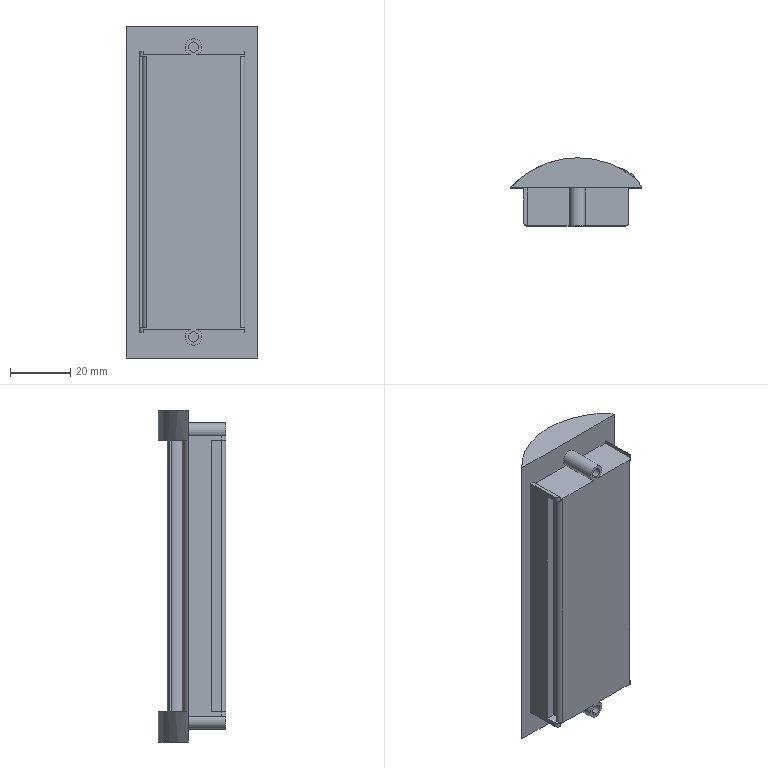Part | SolidWorks | features ICE 3, Extrusion 1, Fillet 1, MirrorPattern 1 | 1 solid | 63 faces | box 43.5 x 22.46 x 110 mm | volume 28533 mm3 | plane 39 | cylinder 24 | commonest cylinder face diameters 3 x6 3.4 x4 5.5 x3 1 x2 15.149 x2 60.026 x2